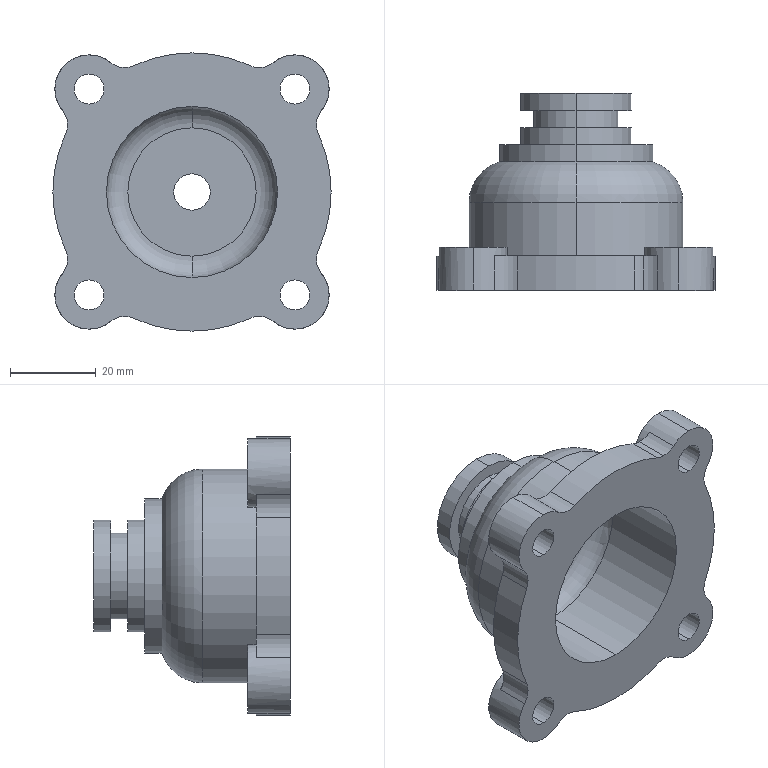Part | SolidWorks | features ICE 3, Chamfer 1, Fillet 1, HoleWzd 1, Revolution 1 | 1 solid | 62 faces | box 65 x 46 x 65 mm | volume 47923 mm3 | cylinder 45 | plane 11 | torus 4 | cone 2 | commonest cylinder face diameters 10 x10 7 x8 16 x8 65 x5 26 x4 8.5 x2